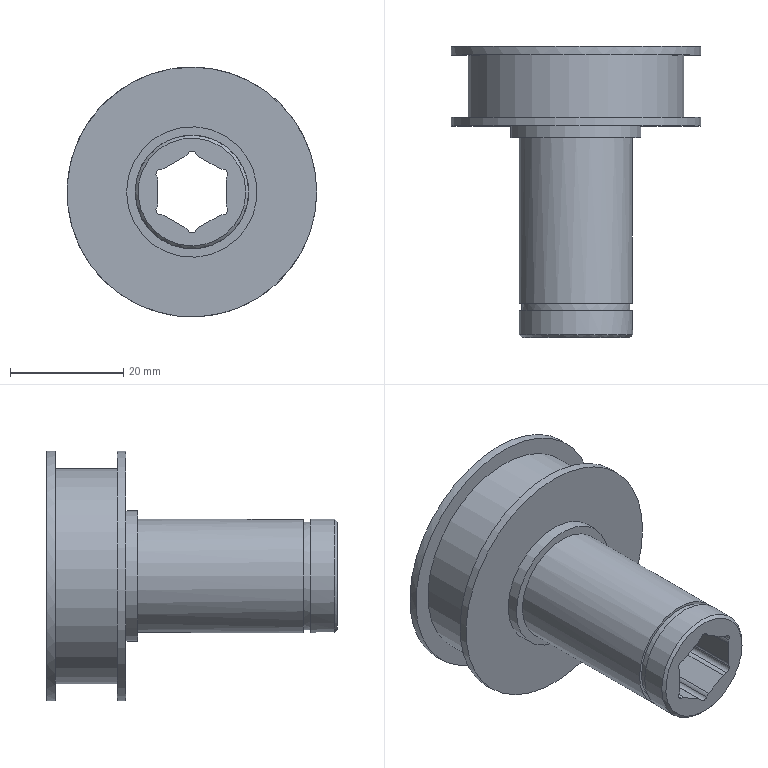Part | STEP file | ROTATION MC_NEW VER-0610_1017 | 1 solid | 40 faces | box 44 x 51.28 x 44 mm | volume 22323 mm3 | cylinder 25 | plane 14 | cone 1 | commonest cylinder face diameters 2.97 x12 1.53 x6 20 x2 44 x2 19 x1 23 x1
STEP:
#1=CARTESIAN_POINT('',(-232.469,307.008,-64.091));
#2=VERTEX_POINT('',#1);
#3=CARTESIAN_POINT('',(-210.469,307.008,-86.091));
#4=VERTEX_POINT('',#3);
#5=CARTESIAN_POINT('',(-232.469,307.008,-86.091));
#6=DIRECTION('',(0.,1.,0.));
#7=DIRECTION('',(0.,0.,1.));
#8=AXIS2_PLACEMENT_3D('',#5,#6,#7);
#9=CIRCLE('',#8,22.);
#10=EDGE_CURVE('',#2,#4,#9,.F.);
#11=ORIENTED_EDGE('',*,*,#10,.F.);
#12=CARTESIAN_POINT('',(-232.469,307.008,-86.091));
#13=DIRECTION('',(0.,1.,0.));
#14=DIRECTION('',(0.,0.,1.));
#15=AXIS2_PLACEMENT_3D('',#12,#13,#14);
#16=CIRCLE('',#15,22.);
#17=EDGE_CURVE('',#4,#2,#16,.F.);
#18=ORIENTED_EDGE('',*,*,#17,.F.);
#19=EDGE_LOOP('',(#11,#18));
#20=FACE_OUTER_BOUND('',#19,.T.);
#21=CARTESIAN_POINT('',(-226.245,307.008,-83.269));
#22=VERTEX_POINT('',#21);
#23=CARTESIAN_POINT('',(-226.454,307.008,-84.029));
#24=VERTEX_POINT('',#23);
#25=CARTESIAN_POINT('',(-224.969,307.008,-84.029));
#26=DIRECTION('',(0.,1.,0.));
#27=DIRECTION('',(-0.9641,0.,0.2654));
#28=AXIS2_PLACEMENT_3D('',#25,#26,#27);
#29=CIRCLE('',#28,1.485);
#30=EDGE_CURVE('',#22,#24,#29,.F.);
#31=ORIENTED_EDGE('',*,*,#30,.F.);
#32=CARTESIAN_POINT('',(-226.913,307.008,-82.112));
#33=VERTEX_POINT('',#32);
#34=CARTESIAN_POINT('',(-226.902,307.008,-82.877));
#35=DIRECTION('',(0.,-1.,0.));
#36=DIRECTION('',(1.,0.,0.));
#37=AXIS2_PLACEMENT_3D('',#34,#35,#36);
#38=CIRCLE('',#37,0.765);
#39=EDGE_CURVE('',#33,#22,#38,.F.);
#40=ORIENTED_EDGE('',*,*,#39,.F.);
#41=CARTESIAN_POINT('',(-227.676,307.008,-81.913));
#42=VERTEX_POINT('',#41);
#43=CARTESIAN_POINT('',(-226.933,307.008,-80.627));
#44=DIRECTION('',(0.,1.,0.));
#45=DIRECTION('',(-0.2522,0.,-0.9677));
#46=AXIS2_PLACEMENT_3D('',#43,#44,#45);
#47=CIRCLE('',#46,1.485);
#48=EDGE_CURVE('',#42,#33,#47,.F.);
#49=ORIENTED_EDGE('',*,*,#48,.F.);
#50=CARTESIAN_POINT('',(-231.248,307.008,-79.851));
#51=VERTEX_POINT('',#50);
#52=CARTESIAN_POINT('',(-227.676,307.008,-81.913));
#53=DIRECTION('',(-0.866,0.,0.5));
#54=VECTOR('',#53,4.125);
#55=LINE('',#52,#54);
#56=EDGE_CURVE('',#51,#42,#55,.F.);
#57=ORIENTED_EDGE('',*,*,#56,.F.);
#58=CARTESIAN_POINT('',(-231.802,307.008,-79.29));
#59=VERTEX_POINT('',#58);
#60=CARTESIAN_POINT('',(-230.506,307.008,-78.565));
#61=DIRECTION('',(0.,1.,0.));
#62=DIRECTION('',(-0.7119,0.,-0.7023));
#63=AXIS2_PLACEMENT_3D('',#60,#61,#62);
#64=CIRCLE('',#63,1.485);
#65=EDGE_CURVE('',#59,#51,#64,.F.);
#66=ORIENTED_EDGE('',*,*,#65,.F.);
#67=CARTESIAN_POINT('',(-233.137,307.008,-79.29));
#68=VERTEX_POINT('',#67);
#69=CARTESIAN_POINT('',(-232.469,307.008,-79.663));
#70=DIRECTION('',(0.,-1.,0.));
#71=DIRECTION('',(1.,0.,0.));
#72=AXIS2_PLACEMENT_3D('',#69,#70,#71);
#73=CIRCLE('',#72,0.765);
#74=EDGE_CURVE('',#68,#59,#73,.F.);
#75=ORIENTED_EDGE('',*,*,#74,.F.);
#76=CARTESIAN_POINT('',(-233.691,307.008,-79.851));
#77=VERTEX_POINT('',#76);
#78=CARTESIAN_POINT('',(-234.433,307.008,-78.565));
#79=DIRECTION('',(0.,1.,0.));
#80=DIRECTION('',(0.7119,0.,-0.7023));
#81=AXIS2_PLACEMENT_3D('',#78,#79,#80);
#82=CIRCLE('',#81,1.485);
#83=EDGE_CURVE('',#77,#68,#82,.F.);
#84=ORIENTED_EDGE('',*,*,#83,.F.);
#85=CARTESIAN_POINT('',(-237.263,307.008,-81.913));
#86=VERTEX_POINT('',#85);
#87=CARTESIAN_POINT('',(-233.691,307.008,-79.851));
#88=DIRECTION('',(-0.866,0.,-0.5));
#89=VECTOR('',#88,4.125);
#90=LINE('',#87,#89);
#91=EDGE_CURVE('',#86,#77,#90,.F.);
#92=ORIENTED_EDGE('',*,*,#91,.F.);
#93=CARTESIAN_POINT('',(-238.026,307.008,-82.112));
#94=VERTEX_POINT('',#93);
#95=CARTESIAN_POINT('',(-238.006,307.008,-80.627));
#96=DIRECTION('',(0.,1.,0.));
#97=DIRECTION('',(0.2522,0.,-0.9677));
#98=AXIS2_PLACEMENT_3D('',#95,#96,#97);
#99=CIRCLE('',#98,1.485);
#100=EDGE_CURVE('',#94,#86,#99,.F.);
#101=ORIENTED_EDGE('',*,*,#100,.F.);
#102=CARTESIAN_POINT('',(-238.694,307.008,-83.269));
#103=VERTEX_POINT('',#102);
#104=CARTESIAN_POINT('',(-238.036,307.008,-82.877));
#105=DIRECTION('',(0.,-1.,0.));
#106=DIRECTION('',(1.,0.,0.));
#107=AXIS2_PLACEMENT_3D('',#104,#105,#106);
#108=CIRCLE('',#107,0.765);
#109=EDGE_CURVE('',#103,#94,#108,.F.);
#110=ORIENTED_EDGE('',*,*,#109,.F.);
#111=CARTESIAN_POINT('',(-238.484,307.008,-84.029));
#112=VERTEX_POINT('',#111);
#113=CARTESIAN_POINT('',(-239.969,307.008,-84.029));
#114=DIRECTION('',(0.,1.,0.));
#115=DIRECTION('',(0.9641,0.,0.2654));
#116=AXIS2_PLACEMENT_3D('',#113,#114,#115);
#117=CIRCLE('',#116,1.485);
#118=EDGE_CURVE('',#112,#103,#117,.F.);
#119=ORIENTED_EDGE('',*,*,#118,.F.);
#120=CARTESIAN_POINT('',(-238.484,307.008,-88.154));
#121=VERTEX_POINT('',#120);
#122=CARTESIAN_POINT('',(-238.484,307.008,-84.029));
#123=DIRECTION('',(0.,0.,-1.));
#124=VECTOR('',#123,4.125);
#125=LINE('',#122,#124);
#126=EDGE_CURVE('',#121,#112,#125,.F.);
#127=ORIENTED_EDGE('',*,*,#126,.F.);
#128=CARTESIAN_POINT('',(-238.694,307.008,-88.914));
#129=VERTEX_POINT('',#128);
#130=CARTESIAN_POINT('',(-239.969,307.008,-88.154));
#131=DIRECTION('',(0.,1.,0.));
#132=DIRECTION('',(0.9641,0.,-0.2654));
#133=AXIS2_PLACEMENT_3D('',#130,#131,#132);
#134=CIRCLE('',#133,1.485);
#135=EDGE_CURVE('',#129,#121,#134,.F.);
#136=ORIENTED_EDGE('',*,*,#135,.F.);
#137=CARTESIAN_POINT('',(-238.026,307.008,-90.07));
#138=VERTEX_POINT('',#137);
#139=CARTESIAN_POINT('',(-238.036,307.008,-89.305));
#140=DIRECTION('',(0.,-1.,0.));
#141=DIRECTION('',(1.,0.,0.));
#142=AXIS2_PLACEMENT_3D('',#139,#140,#141);
#143=CIRCLE('',#142,0.765);
#144=EDGE_CURVE('',#138,#129,#143,.F.);
#145=ORIENTED_EDGE('',*,*,#144,.F.);
#146=CARTESIAN_POINT('',(-237.263,307.008,-90.269));
#147=VERTEX_POINT('',#146);
#148=CARTESIAN_POINT('',(-238.006,307.008,-91.555));
#149=DIRECTION('',(0.,1.,0.));
#150=DIRECTION('',(0.2522,0.,0.9677));
#151=AXIS2_PLACEMENT_3D('',#148,#149,#150);
#152=CIRCLE('',#151,1.485);
#153=EDGE_CURVE('',#147,#138,#152,.F.);
#154=ORIENTED_EDGE('',*,*,#153,.F.);
#155=CARTESIAN_POINT('',(-233.691,307.008,-92.332));
#156=VERTEX_POINT('',#155);
#157=CARTESIAN_POINT('',(-237.263,307.008,-90.269));
#158=DIRECTION('',(0.866,0.,-0.5));
#159=VECTOR('',#158,4.125);
#160=LINE('',#157,#159);
#161=EDGE_CURVE('',#156,#147,#160,.F.);
#162=ORIENTED_EDGE('',*,*,#161,.F.);
#163=CARTESIAN_POINT('',(-233.137,307.008,-92.893));
#164=VERTEX_POINT('',#163);
#165=CARTESIAN_POINT('',(-234.433,307.008,-93.618));
#166=DIRECTION('',(0.,1.,0.));
#167=DIRECTION('',(0.7119,0.,0.7023));
#168=AXIS2_PLACEMENT_3D('',#165,#166,#167);
#169=CIRCLE('',#168,1.485);
#170=EDGE_CURVE('',#164,#156,#169,.F.);
#171=ORIENTED_EDGE('',*,*,#170,.F.);
#172=CARTESIAN_POINT('',(-231.802,307.008,-92.893));
#173=VERTEX_POINT('',#172);
#174=CARTESIAN_POINT('',(-232.469,307.008,-92.519));
#175=DIRECTION('',(0.,-1.,0.));
#176=DIRECTION('',(1.,0.,0.));
#177=AXIS2_PLACEMENT_3D('',#174,#175,#176);
#178=CIRCLE('',#177,0.765);
#179=EDGE_CURVE('',#173,#164,#178,.F.);
#180=ORIENTED_EDGE('',*,*,#179,.F.);
#181=CARTESIAN_POINT('',(-231.248,307.008,-92.332));
#182=VERTEX_POINT('',#181);
#183=CARTESIAN_POINT('',(-230.506,307.008,-93.618));
#184=DIRECTION('',(0.,1.,0.));
#185=DIRECTION('',(-0.7119,0.,0.7023));
#186=AXIS2_PLACEMENT_3D('',#183,#184,#185);
#187=CIRCLE('',#186,1.485);
#188=EDGE_CURVE('',#182,#173,#187,.F.);
#189=ORIENTED_EDGE('',*,*,#188,.F.);
#190=CARTESIAN_POINT('',(-227.676,307.008,-90.269));
#191=VERTEX_POINT('',#190);
#192=CARTESIAN_POINT('',(-231.248,307.008,-92.332));
#193=DIRECTION('',(0.866,0.,0.5));
#194=VECTOR('',#193,4.125);
#195=LINE('',#192,#194);
#196=EDGE_CURVE('',#191,#182,#195,.F.);
#197=ORIENTED_EDGE('',*,*,#196,.F.);
#198=CARTESIAN_POINT('',(-226.913,307.008,-90.07));
#199=VERTEX_POINT('',#198);
#200=CARTESIAN_POINT('',(-226.933,307.008,-91.555));
#201=DIRECTION('',(0.,1.,0.));
#202=DIRECTION('',(-0.2522,0.,0.9677));
#203=AXIS2_PLACEMENT_3D('',#200,#201,#202);
#204=CIRCLE('',#203,1.485);
#205=EDGE_CURVE('',#199,#191,#204,.F.);
#206=ORIENTED_EDGE('',*,*,#205,.F.);
#207=CARTESIAN_POINT('',(-226.245,307.008,-88.914));
#208=VERTEX_POINT('',#207);
#209=CARTESIAN_POINT('',(-226.902,307.008,-89.305));
#210=DIRECTION('',(0.,-1.,0.));
#211=DIRECTION('',(1.,0.,0.));
#212=AXIS2_PLACEMENT_3D('',#209,#210,#211);
#213=CIRCLE('',#212,0.765);
#214=EDGE_CURVE('',#208,#199,#213,.F.);
#215=ORIENTED_EDGE('',*,*,#214,.F.);
#216=CARTESIAN_POINT('',(-226.454,307.008,-88.154));
#217=VERTEX_POINT('',#216);
#218=CARTESIAN_POINT('',(-224.969,307.008,-88.154));
#219=DIRECTION('',(0.,1.,0.));
#220=DIRECTION('',(-0.9641,0.,-0.2654));
#221=AXIS2_PLACEMENT_3D('',#218,#219,#220);
#222=CIRCLE('',#221,1.485);
#223=EDGE_CURVE('',#217,#208,#222,.F.);
#224=ORIENTED_EDGE('',*,*,#223,.F.);
#225=CARTESIAN_POINT('',(-226.454,307.008,-88.154));
#226=DIRECTION('',(0.,0.,1.));
#227=VECTOR('',#226,4.125);
#228=LINE('',#225,#227);
#229=EDGE_CURVE('',#24,#217,#228,.F.);
#230=ORIENTED_EDGE('',*,*,#229,.F.);
#231=EDGE_LOOP('',(#31,#40,#49,#57,#66,#75,#84,#92,#101,#110,#119,#127,#136,#145,#154,#162,#171,#180,#189,#197,#206,#215,#224,#230));
#232=FACE_BOUND('',#231,.T.);
#233=CARTESIAN_POINT('',(-233.469,307.008,-56.281));
#234=DIRECTION('',(0.,1.,0.));
#235=DIRECTION('',(0.,0.,1.));
#236=AXIS2_PLACEMENT_3D('',#233,#234,#235);
#237=PLANE('',#236);
#238=ADVANCED_FACE('',(#20,#232),#237,.T.);
#239=CARTESIAN_POINT('',(-237.263,255.728,-81.913));
#240=VERTEX_POINT('',#239);
#241=CARTESIAN_POINT('',(-237.263,255.728,-81.913));
#242=DIRECTION('',(0.,1.,0.));
#243=VECTOR('',#242,51.28);
#244=LINE('',#241,#243);
#245=EDGE_CURVE('',#86,#240,#244,.F.);
#246=ORIENTED_EDGE('',*,*,#245,.F.);
#247=ORIENTED_EDGE('',*,*,#91,.T.);
#248=CARTESIAN_POINT('',(-233.691,255.728,-79.851));
#249=VERTEX_POINT('',#248);
#250=CARTESIAN_POINT('',(-233.691,307.008,-79.851));
#251=DIRECTION('',(0.,-1.,0.));
#252=VECTOR('',#251,51.28);
#253=LINE('',#250,#252);
#254=EDGE_CURVE('',#249,#77,#253,.F.);
#255=ORIENTED_EDGE('',*,*,#254,.F.);
#256=CARTESIAN_POINT('',(-237.263,255.728,-81.913));
#257=DIRECTION('',(0.866,0.,0.5));
#258=VECTOR('',#257,4.125);
#259=LINE('',#256,#258);
#260=EDGE_CURVE('',#249,#240,#259,.F.);
#261=ORIENTED_EDGE('',*,*,#260,.T.);
#262=EDGE_LOOP('',(#246,#247,#255,#261));
#263=FACE_OUTER_BOUND('',#262,.T.);
#264=CARTESIAN_POINT('',(-235.477,306.008,-80.882));
#265=DIRECTION('',(0.5,0.,-0.866));
#266=DIRECTION('',(-0.866,0.,-0.5));
#267=AXIS2_PLACEMENT_3D('',#264,#265,#266);
#268=PLANE('',#267);
#269=ADVANCED_FACE('',(#263),#268,.T.);
#270=CARTESIAN_POINT('',(-233.137,255.728,-79.29));
#271=VERTEX_POINT('',#270);
#272=CARTESIAN_POINT('',(-233.137,255.728,-79.29));
#273=DIRECTION('',(0.,1.,0.));
#274=VECTOR('',#273,51.28);
#275=LINE('',#272,#274);
#276=EDGE_CURVE('',#68,#271,#275,.F.);
#277=ORIENTED_EDGE('',*,*,#276,.F.);
#278=ORIENTED_EDGE('',*,*,#74,.T.);
#279=CARTESIAN_POINT('',(-231.802,255.728,-79.29));
#280=VERTEX_POINT('',#279);
#281=CARTESIAN_POINT('',(-231.802,307.008,-79.29));
#282=DIRECTION('',(0.,-1.,0.));
#283=VECTOR('',#282,51.28);
#284=LINE('',#281,#283);
#285=EDGE_CURVE('',#280,#59,#284,.F.);
#286=ORIENTED_EDGE('',*,*,#285,.F.);
#287=CARTESIAN_POINT('',(-232.469,255.728,-79.663));
#288=DIRECTION('',(0.,1.,0.));
#289=DIRECTION('',(1.,0.,0.));
#290=AXIS2_PLACEMENT_3D('',#287,#288,#289);
#291=CIRCLE('',#290,0.765);
#292=EDGE_CURVE('',#280,#271,#291,.F.);
#293=ORIENTED_EDGE('',*,*,#292,.T.);
#294=EDGE_LOOP('',(#277,#278,#286,#293));
#295=FACE_OUTER_BOUND('',#294,.T.);
#296=CARTESIAN_POINT('',(-232.469,306.008,-79.663));
#297=DIRECTION('',(0.,1.,0.));
#298=DIRECTION('',(-1.,0.,0.));
#299=AXIS2_PLACEMENT_3D('',#296,#297,#298);
#300=CYLINDRICAL_SURFACE('',#299,0.765);
#301=ADVANCED_FACE('',(#295),#300,.F.);
#302=CARTESIAN_POINT('',(-238.484,255.728,-88.154));
#303=VERTEX_POINT('',#302);
#304=CARTESIAN_POINT('',(-238.484,255.728,-88.154));
#305=DIRECTION('',(0.,1.,0.));
#306=VECTOR('',#305,51.28);
#307=LINE('',#304,#306);
#308=EDGE_CURVE('',#121,#303,#307,.F.);
#309=ORIENTED_EDGE('',*,*,#308,.F.);
#310=ORIENTED_EDGE('',*,*,#126,.T.);
#311=CARTESIAN_POINT('',(-238.484,255.728,-84.029));
#312=VERTEX_POINT('',#311);
#313=CARTESIAN_POINT('',(-238.484,307.008,-84.029));
#314=DIRECTION('',(0.,-1.,0.));
#315=VECTOR('',#314,51.28);
#316=LINE('',#313,#315);
#317=EDGE_CURVE('',#312,#112,#316,.F.);
#318=ORIENTED_EDGE('',*,*,#317,.F.);
#319=CARTESIAN_POINT('',(-238.484,255.728,-88.154));
#320=DIRECTION('',(0.,0.,1.));
#321=VECTOR('',#320,4.125);
#322=LINE('',#319,#321);
#323=EDGE_CURVE('',#312,#303,#322,.F.);
#324=ORIENTED_EDGE('',*,*,#323,.T.);
#325=EDGE_LOOP('',(#309,#310,#318,#324));
#326=FACE_OUTER_BOUND('',#325,.T.);
#327=CARTESIAN_POINT('',(-238.484,306.008,-86.091));
#328=DIRECTION('',(1.,0.,0.));
#329=DIRECTION('',(0.,0.,-1.));
#330=AXIS2_PLACEMENT_3D('',#327,#328,#329);
#331=PLANE('',#330);
#332=ADVANCED_FACE('',(#326),#331,.T.);
#333=CARTESIAN_POINT('',(-231.248,255.728,-79.851));
#334=VERTEX_POINT('',#333);
#335=CARTESIAN_POINT('',(-231.248,255.728,-79.851));
#336=DIRECTION('',(0.,1.,0.));
#337=VECTOR('',#336,51.28);
#338=LINE('',#335,#337);
#339=EDGE_CURVE('',#51,#334,#338,.F.);
#340=ORIENTED_EDGE('',*,*,#339,.F.);
#341=ORIENTED_EDGE('',*,*,#56,.T.);
#342=CARTESIAN_POINT('',(-227.676,255.728,-81.913));
#343=VERTEX_POINT('',#342);
#344=CARTESIAN_POINT('',(-227.676,307.008,-81.913));
#345=DIRECTION('',(0.,-1.,0.));
#346=VECTOR('',#345,51.28);
#347=LINE('',#344,#346);
#348=EDGE_CURVE('',#343,#42,#347,.F.);
#349=ORIENTED_EDGE('',*,*,#348,.F.);
#350=CARTESIAN_POINT('',(-231.248,255.728,-79.851));
#351=DIRECTION('',(0.866,0.,-0.5));
#352=VECTOR('',#351,4.125);
#353=LINE('',#350,#352);
#354=EDGE_CURVE('',#343,#334,#353,.F.);
#355=ORIENTED_EDGE('',*,*,#354,.T.);
#356=EDGE_LOOP('',(#340,#341,#349,#355));
#357=FACE_OUTER_BOUND('',#356,.T.);
#358=CARTESIAN_POINT('',(-229.462,306.008,-80.882));
#359=DIRECTION('',(-0.5,0.,-0.866));
#360=DIRECTION('',(-0.866,0.,0.5));
#361=AXIS2_PLACEMENT_3D('',#358,#359,#360);
#362=PLANE('',#361);
#363=ADVANCED_FACE('',(#357),#362,.T.);
#364=CARTESIAN_POINT('',(-233.691,255.728,-92.332));
#365=VERTEX_POINT('',#364);
#366=CARTESIAN_POINT('',(-233.691,255.728,-92.332));
#367=DIRECTION('',(0.,1.,0.));
#368=VECTOR('',#367,51.28);
#369=LINE('',#366,#368);
#370=EDGE_CURVE('',#156,#365,#369,.F.);
#371=ORIENTED_EDGE('',*,*,#370,.F.);
#372=ORIENTED_EDGE('',*,*,#161,.T.);
#373=CARTESIAN_POINT('',(-237.263,255.728,-90.269));
#374=VERTEX_POINT('',#373);
#375=CARTESIAN_POINT('',(-237.263,307.008,-90.269));
#376=DIRECTION('',(0.,-1.,0.));
#377=VECTOR('',#376,51.28);
#378=LINE('',#375,#377);
#379=EDGE_CURVE('',#374,#147,#378,.F.);
#380=ORIENTED_EDGE('',*,*,#379,.F.);
#381=CARTESIAN_POINT('',(-233.691,255.728,-92.332));
#382=DIRECTION('',(-0.866,0.,0.5));
#383=VECTOR('',#382,4.125);
#384=LINE('',#381,#383);
#385=EDGE_CURVE('',#374,#365,#384,.F.);
#386=ORIENTED_EDGE('',*,*,#385,.T.);
#387=EDGE_LOOP('',(#371,#372,#380,#386));
#388=FACE_OUTER_BOUND('',#387,.T.);
#389=CARTESIAN_POINT('',(-235.477,306.008,-91.3));
#390=DIRECTION('',(0.5,0.,0.866));
#391=DIRECTION('',(0.866,0.,-0.5));
#392=AXIS2_PLACEMENT_3D('',#389,#390,#391);
#393=PLANE('',#392);
#394=ADVANCED_FACE('',(#388),#393,.T.);
#395=CARTESIAN_POINT('',(-226.454,255.728,-84.029));
#396=VERTEX_POINT('',#395);
#397=CARTESIAN_POINT('',(-226.454,255.728,-84.029));
#398=DIRECTION('',(0.,1.,0.));
#399=VECTOR('',#398,51.28);
#400=LINE('',#397,#399);
#401=EDGE_CURVE('',#24,#396,#400,.F.);
#402=ORIENTED_EDGE('',*,*,#401,.F.);
#403=ORIENTED_EDGE('',*,*,#229,.T.);
#404=CARTESIAN_POINT('',(-226.454,255.728,-88.154));
#405=VERTEX_POINT('',#404);
#406=CARTESIAN_POINT('',(-226.454,307.008,-88.154));
#407=DIRECTION('',(0.,-1.,0.));
#408=VECTOR('',#407,51.28);
#409=LINE('',#406,#408);
#410=EDGE_CURVE('',#405,#217,#409,.F.);
#411=ORIENTED_EDGE('',*,*,#410,.F.);
#412=CARTESIAN_POINT('',(-226.454,255.728,-84.029));
#413=DIRECTION('',(0.,0.,-1.));
#414=VECTOR('',#413,4.125);
#415=LINE('',#412,#414);
#416=EDGE_CURVE('',#405,#396,#415,.F.);
#417=ORIENTED_EDGE('',*,*,#416,.T.);
#418=EDGE_LOOP('',(#402,#403,#411,#417));
#419=FACE_OUTER_BOUND('',#418,.T.);
#420=CARTESIAN_POINT('',(-226.454,306.008,-86.091));
#421=DIRECTION('',(-1.,0.,0.));
#422=DIRECTION('',(0.,0.,1.));
#423=AXIS2_PLACEMENT_3D('',#420,#421,#422);
#424=PLANE('',#423);
#425=ADVANCED_FACE('',(#419),#424,.T.);
#426=CARTESIAN_POINT('',(-231.802,255.728,-92.893));
#427=VERTEX_POINT('',#426);
#428=CARTESIAN_POINT('',(-231.802,255.728,-92.893));
#429=DIRECTION('',(0.,1.,0.));
#430=VECTOR('',#429,51.28);
#431=LINE('',#428,#430);
#432=EDGE_CURVE('',#173,#427,#431,.F.);
#433=ORIENTED_EDGE('',*,*,#432,.F.);
#434=ORIENTED_EDGE('',*,*,#179,.T.);
#435=CARTESIAN_POINT('',(-233.137,255.728,-92.893));
#436=VERTEX_POINT('',#435);
#437=CARTESIAN_POINT('',(-233.137,307.008,-92.893));
#438=DIRECTION('',(0.,-1.,0.));
#439=VECTOR('',#438,51.28);
#440=LINE('',#437,#439);
#441=EDGE_CURVE('',#436,#164,#440,.F.);
#442=ORIENTED_EDGE('',*,*,#441,.F.);
#443=CARTESIAN_POINT('',(-232.469,255.728,-92.519));
#444=DIRECTION('',(0.,1.,0.));
#445=DIRECTION('',(1.,0.,0.));
#446=AXIS2_PLACEMENT_3D('',#443,#444,#445);
#447=CIRCLE('',#446,0.765);
#448=EDGE_CURVE('',#436,#427,#447,.F.);
#449=ORIENTED_EDGE('',*,*,#448,.T.);
#450=EDGE_LOOP('',(#433,#434,#442,#449));
#451=FACE_OUTER_BOUND('',#450,.T.);
#452=CARTESIAN_POINT('',(-232.469,306.008,-92.519));
#453=DIRECTION('',(0.,1.,0.));
#454=DIRECTION('',(-1.,0.,0.));
#455=AXIS2_PLACEMENT_3D('',#452,#453,#454);
#456=CYLINDRICAL_SURFACE('',#455,0.765);
#457=ADVANCED_FACE('',(#451),#456,.F.);
#458=CARTESIAN_POINT('',(-227.676,255.728,-90.269));
#459=VERTEX_POINT('',#458);
#460=CARTESIAN_POINT('',(-227.676,255.728,-90.269));
#461=DIRECTION('',(0.,1.,0.));
#462=VECTOR('',#461,51.28);
#463=LINE('',#460,#462);
#464=EDGE_CURVE('',#191,#459,#463,.F.);
#465=ORIENTED_EDGE('',*,*,#464,.F.);
#466=ORIENTED_EDGE('',*,*,#196,.T.);
#467=CARTESIAN_POINT('',(-231.248,255.728,-92.332));
#468=VERTEX_POINT('',#467);
#469=CARTESIAN_POINT('',(-231.248,307.008,-92.332));
#470=DIRECTION('',(0.,-1.,0.));
#471=VECTOR('',#470,51.28);
#472=LINE('',#469,#471);
#473=EDGE_CURVE('',#468,#182,#472,.F.);
#474=ORIENTED_EDGE('',*,*,#473,.F.);
#475=CARTESIAN_POINT('',(-227.676,255.728,-90.269));
#476=DIRECTION('',(-0.866,0.,-0.5));
#477=VECTOR('',#476,4.125);
#478=LINE('',#475,#477);
#479=EDGE_CURVE('',#468,#459,#478,.F.);
#480=ORIENTED_EDGE('',*,*,#479,.T.);
#481=EDGE_LOOP('',(#465,#466,#474,#480));
#482=FACE_OUTER_BOUND('',#481,.T.);
#483=CARTESIAN_POINT('',(-229.462,306.008,-91.3));
#484=DIRECTION('',(-0.5,0.,0.866));
#485=DIRECTION('',(0.866,0.,0.5));
#486=AXIS2_PLACEMENT_3D('',#483,#484,#485);
#487=PLANE('',#486);
#488=ADVANCED_FACE('',(#482),#487,.T.);
#489=CARTESIAN_POINT('',(-243.969,290.968,-86.091));
#490=VERTEX_POINT('',#489);
#491=CARTESIAN_POINT('',(-232.469,290.968,-86.091));
#492=DIRECTION('',(0.,-1.,0.));
#493=DIRECTION('',(-1.,0.,0.));
#494=AXIS2_PLACEMENT_3D('',#491,#492,#493);
#495=CIRCLE('',#494,11.5);
#496=EDGE_CURVE('',#490,#490,#495,.F.);
#497=ORIENTED_EDGE('',*,*,#496,.F.);
#498=EDGE_LOOP('',(#497));
#499=FACE_OUTER_BOUND('',#498,.T.);
#500=CARTESIAN_POINT('',(-232.469,290.968,-76.091));
#501=VERTEX_POINT('',#500);
#502=CARTESIAN_POINT('',(-242.469,290.968,-86.091));
#503=VERTEX_POINT('',#502);
#504=CARTESIAN_POINT('',(-232.469,290.968,-86.091));
#505=DIRECTION('',(0.,-1.,0.));
#506=DIRECTION('',(0.,0.,1.));
#507=AXIS2_PLACEMENT_3D('',#504,#505,#506);
#508=CIRCLE('',#507,10.);
#509=EDGE_CURVE('',#501,#503,#508,.F.);
#510=ORIENTED_EDGE('',*,*,#509,.T.);
#511=CARTESIAN_POINT('',(-232.469,290.968,-86.091));
#512=DIRECTION('',(0.,-1.,0.));
#513=DIRECTION('',(0.,0.,1.));
#514=AXIS2_PLACEMENT_3D('',#511,#512,#513);
#515=CIRCLE('',#514,10.);
#516=EDGE_CURVE('',#503,#501,#515,.F.);
#517=ORIENTED_EDGE('',*,*,#516,.T.);
#518=EDGE_LOOP('',(#510,#517));
#519=FACE_BOUND('',#518,.T.);
#520=CARTESIAN_POINT('',(-233.469,290.968,-56.281));
#521=DIRECTION('',(0.,1.,0.));
#522=DIRECTION('',(0.,0.,1.));
#523=AXIS2_PLACEMENT_3D('',#520,#521,#522);
#524=PLANE('',#523);
#525=ADVANCED_FACE('',(#499,#519),#524,.F.);
#526=CARTESIAN_POINT('',(-232.469,293.008,-64.091));
#527=VERTEX_POINT('',#526);
#528=CARTESIAN_POINT('',(-210.469,293.008,-86.091));
#529=VERTEX_POINT('',#528);
#530=CARTESIAN_POINT('',(-232.469,293.008,-86.091));
#531=DIRECTION('',(0.,-1.,0.));
#532=DIRECTION('',(0.,0.,1.));
#533=AXIS2_PLACEMENT_3D('',#530,#531,#532);
#534=CIRCLE('',#533,22.);
#535=EDGE_CURVE('',#527,#529,#534,.F.);
#536=ORIENTED_EDGE('',*,*,#535,.F.);
#537=CARTESIAN_POINT('',(-232.469,293.008,-86.091));
#538=DIRECTION('',(0.,-1.,0.));
#539=DIRECTION('',(0.,0.,1.));
#540=AXIS2_PLACEMENT_3D('',#537,#538,#539);
#541=CIRCLE('',#540,22.);
#542=EDGE_CURVE('',#529,#527,#541,.F.);
#543=ORIENTED_EDGE('',*,*,#542,.F.);
#544=EDGE_LOOP('',(#536,#543));
#545=FACE_OUTER_BOUND('',#544,.T.);
#546=CARTESIAN_POINT('',(-243.969,293.008,-86.091));
#547=VERTEX_POINT('',#546);
#548=CARTESIAN_POINT('',(-232.469,293.008,-86.091));
#549=DIRECTION('',(0.,-1.,0.));
#550=DIRECTION('',(-1.,0.,0.));
#551=AXIS2_PLACEMENT_3D('',#548,#549,#550);
#552=CIRCLE('',#551,11.5);
#553=EDGE_CURVE('',#547,#547,#552,.F.);
#554=ORIENTED_EDGE('',*,*,#553,.T.);
#555=EDGE_LOOP('',(#554));
#556=FACE_BOUND('',#555,.T.);
#557=CARTESIAN_POINT('',(-233.469,293.008,-56.281));
#558=DIRECTION('',(0.,1.,0.));
#559=DIRECTION('',(0.,0.,1.));
#560=AXIS2_PLACEMENT_3D('',#557,#558,#559);
#561=PLANE('',#560);
#562=ADVANCED_FACE('',(#545,#556),#561,.F.);
#563=CARTESIAN_POINT('',(-232.469,305.508,-108.091));
#564=VERTEX_POINT('',#563);
#565=CARTESIAN_POINT('',(-210.469,305.508,-86.091));
#566=VERTEX_POINT('',#565);
#567=CARTESIAN_POINT('',(-232.469,305.508,-86.091));
#568=DIRECTION('',(0.,-1.,0.));
#569=DIRECTION('',(0.,0.,-1.));
#570=AXIS2_PLACEMENT_3D('',#567,#568,#569);
#571=CIRCLE('',#570,22.);
#572=EDGE_CURVE('',#564,#566,#571,.F.);
#573=ORIENTED_EDGE('',*,*,#572,.F.);
#574=CARTESIAN_POINT('',(-232.469,305.508,-86.091));
#575=DIRECTION('',(0.,-1.,0.));
#576=DIRECTION('',(0.,0.,-1.));
#577=AXIS2_PLACEMENT_3D('',#574,#575,#576);
#578=CIRCLE('',#577,22.);
#579=EDGE_CURVE('',#566,#564,#578,.F.);
#580=ORIENTED_EDGE('',*,*,#579,.F.);
#581=EDGE_LOOP('',(#573,#580));
#582=FACE_OUTER_BOUND('',#581,.T.);
#583=CARTESIAN_POINT('',(-232.469,305.508,-105.091));
#584=VERTEX_POINT('',#583);
#585=CARTESIAN_POINT('',(-213.469,305.508,-86.091));
#586=VERTEX_POINT('',#585);
#587=CARTESIAN_POINT('',(-232.469,305.508,-86.091));
#588=DIRECTION('',(0.,1.,0.));
#589=DIRECTION('',(0.,0.,-1.));
#590=AXIS2_PLACEMENT_3D('',#587,#588,#589);
#591=CIRCLE('',#590,19.);
#592=EDGE_CURVE('',#584,#586,#591,.F.);
#593=ORIENTED_EDGE('',*,*,#592,.F.);
#594=CARTESIAN_POINT('',(-232.469,305.508,-86.091));
#595=DIRECTION('',(0.,1.,0.));
#596=DIRECTION('',(0.,0.,-1.));
#597=AXIS2_PLACEMENT_3D('',#594,#595,#596);
#598=CIRCLE('',#597,19.);
#599=EDGE_CURVE('',#586,#584,#598,.F.);
#600=ORIENTED_EDGE('',*,*,#599,.F.);
#601=EDGE_LOOP('',(#593,#600));
#602=FACE_BOUND('',#601,.T.);
#603=CARTESIAN_POINT('',(-212.469,305.508,-86.091));
#604=DIRECTION('',(0.,-1.,0.));
#605=DIRECTION('',(0.,0.,-1.));
#606=AXIS2_PLACEMENT_3D('',#603,#604,#605);
#607=PLANE('',#606);
#608=ADVANCED_FACE('',(#582,#602),#607,.T.);
#609=CARTESIAN_POINT('',(-232.469,294.508,-64.091));
#610=VERTEX_POINT('',#609);
#611=CARTESIAN_POINT('',(-210.469,294.508,-86.091));
#612=VERTEX_POINT('',#611);
#613=CARTESIAN_POINT('',(-232.469,294.508,-86.091));
#614=DIRECTION('',(0.,1.,0.));
#615=DIRECTION('',(0.,0.,1.));
#616=AXIS2_PLACEMENT_3D('',#613,#614,#615);
#617=CIRCLE('',#616,22.);
#618=EDGE_CURVE('',#610,#612,#617,.F.);
#619=ORIENTED_EDGE('',*,*,#618,.F.);
#620=CARTESIAN_POINT('',(-232.469,294.508,-86.091));
#621=DIRECTION('',(0.,1.,0.));
#622=DIRECTION('',(0.,0.,1.));
#623=AXIS2_PLACEMENT_3D('',#620,#621,#622);
#624=CIRCLE('',#623,22.);
#625=EDGE_CURVE('',#612,#610,#624,.F.);
#626=ORIENTED_EDGE('',*,*,#625,.F.);
#627=EDGE_LOOP('',(#619,#626));
#628=FACE_OUTER_BOUND('',#627,.T.);
#629=CARTESIAN_POINT('',(-232.469,294.508,-105.091));
#630=VERTEX_POINT('',#629);
#631=CARTESIAN_POINT('',(-213.469,294.508,-86.091));
#632=VERTEX_POINT('',#631);
#633=CARTESIAN_POINT('',(-232.469,294.508,-86.091));
#634=DIRECTION('',(0.,-1.,0.));
#635=DIRECTION('',(0.,0.,1.));
#636=AXIS2_PLACEMENT_3D('',#633,#634,#635);
#637=CIRCLE('',#636,19.);
#638=EDGE_CURVE('',#630,#632,#637,.F.);
#639=ORIENTED_EDGE('',*,*,#638,.F.);
#640=CARTESIAN_POINT('',(-232.469,294.508,-86.091));
#641=DIRECTION('',(0.,-1.,0.));
#642=DIRECTION('',(0.,0.,1.));
#643=AXIS2_PLACEMENT_3D('',#640,#641,#642);
#644=CIRCLE('',#643,19.);
#645=EDGE_CURVE('',#632,#630,#644,.F.);
#646=ORIENTED_EDGE('',*,*,#645,.F.);
#647=EDGE_LOOP('',(#639,#646));
#648=FACE_BOUND('',#647,.T.);
#649=CARTESIAN_POINT('',(-212.469,294.508,-86.091));
#650=DIRECTION('',(0.,1.,0.));
#651=DIRECTION('',(0.,0.,1.));
#652=AXIS2_PLACEMENT_3D('',#649,#650,#651);
#653=PLANE('',#652);
#654=ADVANCED_FACE('',(#628,#648),#653,.T.);
#655=CARTESIAN_POINT('',(-232.469,261.768,-96.091));
#656=VERTEX_POINT('',#655);
#657=CARTESIAN_POINT('',(-242.469,261.768,-86.091));
#658=VERTEX_POINT('',#657);
#659=CARTESIAN_POINT('',(-232.469,261.768,-86.091));
#660=DIRECTION('',(0.,1.,0.));
#661=DIRECTION('',(0.,0.,-1.));
#662=AXIS2_PLACEMENT_3D('',#659,#660,#661);
#663=CIRCLE('',#662,10.);
#664=EDGE_CURVE('',#656,#658,#663,.F.);
#665=ORIENTED_EDGE('',*,*,#664,.T.);
#666=CARTESIAN_POINT('',(-232.469,261.768,-86.091));
#667=DIRECTION('',(0.,1.,0.));
#668=DIRECTION('',(0.,0.,-1.));
#669=AXIS2_PLACEMENT_3D('',#666,#667,#668);
#670=CIRCLE('',#669,10.);
#671=EDGE_CURVE('',#658,#656,#670,.F.);
#672=ORIENTED_EDGE('',*,*,#671,.T.);
#673=EDGE_LOOP('',(#665,#672));
#674=FACE_OUTER_BOUND('',#673,.T.);
#675=CARTESIAN_POINT('',(-232.469,261.768,-95.591));
#676=VERTEX_POINT('',#675);
#677=CARTESIAN_POINT('',(-241.969,261.768,-86.091));
#678=VERTEX_POINT('',#677);
#679=CARTESIAN_POINT('',(-232.469,261.768,-86.091));
#680=DIRECTION('',(0.,1.,0.));
#681=DIRECTION('',(0.,0.,-1.));
#682=AXIS2_PLACEMENT_3D('',#679,#680,#681);
#683=CIRCLE('',#682,9.5);
#684=EDGE_CURVE('',#676,#678,#683,.F.);
#685=ORIENTED_EDGE('',*,*,#684,.F.);
#686=CARTESIAN_POINT('',(-232.469,261.768,-86.091));
#687=DIRECTION('',(0.,1.,0.));
#688=DIRECTION('',(0.,0.,-1.));
#689=AXIS2_PLACEMENT_3D('',#686,#687,#688);
#690=CIRCLE('',#689,9.5);
#691=EDGE_CURVE('',#678,#676,#690,.F.);
#692=ORIENTED_EDGE('',*,*,#691,.F.);
#693=EDGE_LOOP('',(#685,#692));
#694=FACE_BOUND('',#693,.T.);
#695=CARTESIAN_POINT('',(-242.469,261.768,-86.091));
#696=DIRECTION('',(0.,-1.,0.));
#697=DIRECTION('',(0.,0.,-1.));
#698=AXIS2_PLACEMENT_3D('',#695,#696,#697);
#699=PLANE('',#698);
#700=ADVANCED_FACE('',(#674,#694),#699,.T.);
#701=CARTESIAN_POINT('',(-232.469,260.468,-76.091));
#702=VERTEX_POINT('',#701);
#703=CARTESIAN_POINT('',(-242.469,260.468,-86.091));
#704=VERTEX_POINT('',#703);
#705=CARTESIAN_POINT('',(-232.469,260.468,-86.091));
#706=DIRECTION('',(0.,1.,0.));
#707=DIRECTION('',(0.,0.,1.));
#708=AXIS2_PLACEMENT_3D('',#705,#706,#707);
#709=CIRCLE('',#708,10.);
#710=EDGE_CURVE('',#702,#704,#709,.F.);
#711=ORIENTED_EDGE('',*,*,#710,.F.);
#712=CARTESIAN_POINT('',(-232.469,260.468,-86.091));
#713=DIRECTION('',(0.,1.,0.));
#714=DIRECTION('',(0.,0.,1.));
#715=AXIS2_PLACEMENT_3D('',#712,#713,#714);
#716=CIRCLE('',#715,10.);
#717=EDGE_CURVE('',#704,#702,#716,.F.);
#718=ORIENTED_EDGE('',*,*,#717,.F.);
#719=EDGE_LOOP('',(#711,#718));
#720=FACE_OUTER_BOUND('',#719,.T.);
#721=CARTESIAN_POINT('',(-232.469,260.468,-76.591));
#722=VERTEX_POINT('',#721);
#723=CARTESIAN_POINT('',(-241.969,260.468,-86.091));
#724=VERTEX_POINT('',#723);
#725=CARTESIAN_POINT('',(-232.469,260.468,-86.091));
#726=DIRECTION('',(0.,1.,0.));
#727=DIRECTION('',(0.,0.,1.));
#728=AXIS2_PLACEMENT_3D('',#725,#726,#727);
#729=CIRCLE('',#728,9.5);
#730=EDGE_CURVE('',#722,#724,#729,.F.);
#731=ORIENTED_EDGE('',*,*,#730,.T.);
#732=CARTESIAN_POINT('',(-232.469,260.468,-86.091));
#733=DIRECTION('',(0.,1.,0.));
#734=DIRECTION('',(0.,0.,1.));
#735=AXIS2_PLACEMENT_3D('',#732,#733,#734);
#736=CIRCLE('',#735,9.5);
#737=EDGE_CURVE('',#724,#722,#736,.F.);
#738=ORIENTED_EDGE('',*,*,#737,.T.);
#739=EDGE_LOOP('',(#731,#738));
#740=FACE_BOUND('',#739,.T.);
#741=CARTESIAN_POINT('',(-242.469,260.468,-86.091));
#742=DIRECTION('',(0.,1.,0.));
#743=DIRECTION('',(0.,0.,1.));
#744=AXIS2_PLACEMENT_3D('',#741,#742,#743);
#745=PLANE('',#744);
#746=ADVANCED_FACE('',(#720,#740),#745,.T.);
#747=CARTESIAN_POINT('',(-232.469,255.728,-95.591));
#748=VERTEX_POINT('',#747);
#749=CARTESIAN_POINT('',(-222.969,255.728,-86.091));
#750=VERTEX_POINT('',#749);
#751=CARTESIAN_POINT('',(-232.469,255.728,-86.091));
#752=DIRECTION('',(0.,-1.,0.));
#753=DIRECTION('',(0.,0.,-1.));
#754=AXIS2_PLACEMENT_3D('',#751,#752,#753);
#755=CIRCLE('',#754,9.5);
#756=EDGE_CURVE('',#748,#750,#755,.F.);
#757=ORIENTED_EDGE('',*,*,#756,.F.);
#758=CARTESIAN_POINT('',(-232.469,255.728,-86.091));
#759=DIRECTION('',(0.,-1.,0.));
#760=DIRECTION('',(0.,0.,-1.));
#761=AXIS2_PLACEMENT_3D('',#758,#759,#760);
#762=CIRCLE('',#761,9.5);
#763=EDGE_CURVE('',#750,#748,#762,.F.);
#764=ORIENTED_EDGE('',*,*,#763,.F.);
#765=EDGE_LOOP('',(#757,#764));
#766=FACE_OUTER_BOUND('',#765,.T.);
#767=CARTESIAN_POINT('',(-238.694,255.728,-88.914));
#768=VERTEX_POINT('',#767);
#769=CARTESIAN_POINT('',(-238.026,255.728,-90.07));
#770=VERTEX_POINT('',#769);
#771=CARTESIAN_POINT('',(-238.036,255.728,-89.305));
#772=DIRECTION('',(0.,1.,0.));
#773=DIRECTION('',(1.,0.,0.));
#774=AXIS2_PLACEMENT_3D('',#771,#772,#773);
#775=CIRCLE('',#774,0.765);
#776=EDGE_CURVE('',#768,#770,#775,.F.);
#777=ORIENTED_EDGE('',*,*,#776,.F.);
#778=CARTESIAN_POINT('',(-239.969,255.728,-88.154));
#779=DIRECTION('',(0.,-1.,0.));
#780=DIRECTION('',(0.9641,0.,-0.2654));
#781=AXIS2_PLACEMENT_3D('',#778,#779,#780);
#782=CIRCLE('',#781,1.485);
#783=EDGE_CURVE('',#303,#768,#782,.F.);
#784=ORIENTED_EDGE('',*,*,#783,.F.);
#785=ORIENTED_EDGE('',*,*,#323,.F.);
#786=CARTESIAN_POINT('',(-238.694,255.728,-83.269));
#787=VERTEX_POINT('',#786);
#788=CARTESIAN_POINT('',(-239.969,255.728,-84.029));
#789=DIRECTION('',(0.,-1.,0.));
#790=DIRECTION('',(0.9641,0.,0.2654));
#791=AXIS2_PLACEMENT_3D('',#788,#789,#790);
#792=CIRCLE('',#791,1.485);
#793=EDGE_CURVE('',#787,#312,#792,.F.);
#794=ORIENTED_EDGE('',*,*,#793,.F.);
#795=CARTESIAN_POINT('',(-238.026,255.728,-82.112));
#796=VERTEX_POINT('',#795);
#797=CARTESIAN_POINT('',(-238.036,255.728,-82.877));
#798=DIRECTION('',(0.,1.,0.));
#799=DIRECTION('',(1.,0.,0.));
#800=AXIS2_PLACEMENT_3D('',#797,#798,#799);
#801=CIRCLE('',#800,0.765);
#802=EDGE_CURVE('',#796,#787,#801,.F.);
#803=ORIENTED_EDGE('',*,*,#802,.F.);
#804=CARTESIAN_POINT('',(-238.006,255.728,-80.627));
#805=DIRECTION('',(0.,-1.,0.));
#806=DIRECTION('',(0.2522,0.,-0.9677));
#807=AXIS2_PLACEMENT_3D('',#804,#805,#806);
#808=CIRCLE('',#807,1.485);
#809=EDGE_CURVE('',#240,#796,#808,.F.);
#810=ORIENTED_EDGE('',*,*,#809,.F.);
#811=ORIENTED_EDGE('',*,*,#260,.F.);
#812=CARTESIAN_POINT('',(-234.433,255.728,-78.565));
#813=DIRECTION('',(0.,-1.,0.));
#814=DIRECTION('',(0.7119,0.,-0.7023));
#815=AXIS2_PLACEMENT_3D('',#812,#813,#814);
#816=CIRCLE('',#815,1.485);
#817=EDGE_CURVE('',#271,#249,#816,.F.);
#818=ORIENTED_EDGE('',*,*,#817,.F.);
#819=ORIENTED_EDGE('',*,*,#292,.F.);
#820=CARTESIAN_POINT('',(-230.506,255.728,-78.565));
#821=DIRECTION('',(0.,-1.,0.));
#822=DIRECTION('',(-0.7119,0.,-0.7023));
#823=AXIS2_PLACEMENT_3D('',#820,#821,#822);
#824=CIRCLE('',#823,1.485);
#825=EDGE_CURVE('',#334,#280,#824,.F.);
#826=ORIENTED_EDGE('',*,*,#825,.F.);
#827=ORIENTED_EDGE('',*,*,#354,.F.);
#828=CARTESIAN_POINT('',(-226.913,255.728,-82.112));
#829=VERTEX_POINT('',#828);
#830=CARTESIAN_POINT('',(-226.933,255.728,-80.627));
#831=DIRECTION('',(0.,-1.,0.));
#832=DIRECTION('',(-0.2522,0.,-0.9677));
#833=AXIS2_PLACEMENT_3D('',#830,#831,#832);
#834=CIRCLE('',#833,1.485);
#835=EDGE_CURVE('',#829,#343,#834,.F.);
#836=ORIENTED_EDGE('',*,*,#835,.F.);
#837=CARTESIAN_POINT('',(-226.245,255.728,-83.269));
#838=VERTEX_POINT('',#837);
#839=CARTESIAN_POINT('',(-226.902,255.728,-82.877));
#840=DIRECTION('',(0.,1.,0.));
#841=DIRECTION('',(1.,0.,0.));
#842=AXIS2_PLACEMENT_3D('',#839,#840,#841);
#843=CIRCLE('',#842,0.765);
#844=EDGE_CURVE('',#838,#829,#843,.F.);
#845=ORIENTED_EDGE('',*,*,#844,.F.);
#846=CARTESIAN_POINT('',(-224.969,255.728,-84.029));
#847=DIRECTION('',(0.,-1.,0.));
#848=DIRECTION('',(-0.9641,0.,0.2654));
#849=AXIS2_PLACEMENT_3D('',#846,#847,#848);
#850=CIRCLE('',#849,1.485);
#851=EDGE_CURVE('',#396,#838,#850,.F.);
#852=ORIENTED_EDGE('',*,*,#851,.F.);
#853=ORIENTED_EDGE('',*,*,#416,.F.);
#854=CARTESIAN_POINT('',(-226.245,255.728,-88.914));
#855=VERTEX_POINT('',#854);
#856=CARTESIAN_POINT('',(-224.969,255.728,-88.154));
#857=DIRECTION('',(0.,-1.,0.));
#858=DIRECTION('',(-0.9641,0.,-0.2654));
#859=AXIS2_PLACEMENT_3D('',#856,#857,#858);
#860=CIRCLE('',#859,1.485);
#861=EDGE_CURVE('',#855,#405,#860,.F.);
#862=ORIENTED_EDGE('',*,*,#861,.F.);
#863=CARTESIAN_POINT('',(-226.913,255.728,-90.07));
#864=VERTEX_POINT('',#863);
#865=CARTESIAN_POINT('',(-226.902,255.728,-89.305));
#866=DIRECTION('',(0.,1.,0.));
#867=DIRECTION('',(1.,0.,0.));
#868=AXIS2_PLACEMENT_3D('',#865,#866,#867);
#869=CIRCLE('',#868,0.765);
#870=EDGE_CURVE('',#864,#855,#869,.F.);
#871=ORIENTED_EDGE('',*,*,#870,.F.);
#872=CARTESIAN_POINT('',(-226.933,255.728,-91.555));
#873=DIRECTION('',(0.,-1.,0.));
#874=DIRECTION('',(-0.2522,0.,0.9677));
#875=AXIS2_PLACEMENT_3D('',#872,#873,#874);
#876=CIRCLE('',#875,1.485);
#877=EDGE_CURVE('',#459,#864,#876,.F.);
#878=ORIENTED_EDGE('',*,*,#877,.F.);
#879=ORIENTED_EDGE('',*,*,#479,.F.);
#880=CARTESIAN_POINT('',(-230.506,255.728,-93.618));
#881=DIRECTION('',(0.,-1.,0.));
#882=DIRECTION('',(-0.7119,0.,0.7023));
#883=AXIS2_PLACEMENT_3D('',#880,#881,#882);
#884=CIRCLE('',#883,1.485);
#885=EDGE_CURVE('',#427,#468,#884,.F.);
#886=ORIENTED_EDGE('',*,*,#885,.F.);
#887=ORIENTED_EDGE('',*,*,#448,.F.);
#888=CARTESIAN_POINT('',(-234.433,255.728,-93.618));
#889=DIRECTION('',(0.,-1.,0.));
#890=DIRECTION('',(0.7119,0.,0.7023));
#891=AXIS2_PLACEMENT_3D('',#888,#889,#890);
#892=CIRCLE('',#891,1.485);
#893=EDGE_CURVE('',#365,#436,#892,.F.);
#894=ORIENTED_EDGE('',*,*,#893,.F.);
#895=ORIENTED_EDGE('',*,*,#385,.F.);
#896=CARTESIAN_POINT('',(-238.006,255.728,-91.555));
#897=DIRECTION('',(0.,-1.,0.));
#898=DIRECTION('',(0.2522,0.,0.9677));
#899=AXIS2_PLACEMENT_3D('',#896,#897,#898);
#900=CIRCLE('',#899,1.485);
#901=EDGE_CURVE('',#770,#374,#900,.F.);
#902=ORIENTED_EDGE('',*,*,#901,.F.);
#903=EDGE_LOOP('',(#777,#784,#785,#794,#803,#810,#811,#818,#819,#826,#827,#836,#845,#852,#853,#862,#871,#878,#879,#886,#887,#894,#895,#902));
#904=FACE_BOUND('',#903,.T.);
#905=CARTESIAN_POINT('',(-232.469,255.728,-86.091));
#906=DIRECTION('',(0.,-1.,0.));
#907=DIRECTION('',(0.,0.,-1.));
#908=AXIS2_PLACEMENT_3D('',#905,#906,#907);
#909=PLANE('',#908);
#910=ADVANCED_FACE('',(#766,#904),#909,.T.);
#911=ORIENTED_EDGE('',*,*,#205,.T.);
#912=ORIENTED_EDGE('',*,*,#464,.T.);
#913=ORIENTED_EDGE('',*,*,#877,.T.);
#914=CARTESIAN_POINT('',(-226.913,307.008,-90.07));
#915=DIRECTION('',(0.,-1.,0.));
#916=VECTOR('',#915,51.28);
#917=LINE('',#914,#916);
#918=EDGE_CURVE('',#864,#199,#917,.F.);
#919=ORIENTED_EDGE('',*,*,#918,.T.);
#920=EDGE_LOOP('',(#911,#912,#913,#919));
#921=FACE_OUTER_BOUND('',#920,.T.);
#922=CARTESIAN_POINT('',(-226.933,306.008,-91.555));
#923=DIRECTION('',(0.,1.,0.));
#924=DIRECTION('',(-0.2522,0.,0.9677));
#925=AXIS2_PLACEMENT_3D('',#922,#923,#924);
#926=CYLINDRICAL_SURFACE('',#925,1.485);
#927=ADVANCED_FACE('',(#921),#926,.T.);
#928=ORIENTED_EDGE('',*,*,#885,.T.);
#929=ORIENTED_EDGE('',*,*,#473,.T.);
#930=ORIENTED_EDGE('',*,*,#188,.T.);
#931=ORIENTED_EDGE('',*,*,#432,.T.);
#932=EDGE_LOOP('',(#928,#929,#930,#931));
#933=FACE_OUTER_BOUND('',#932,.T.);
#934=CARTESIAN_POINT('',(-230.506,306.008,-93.618));
#935=DIRECTION('',(0.,-1.,0.));
#936=DIRECTION('',(-0.7119,0.,0.7023));
#937=AXIS2_PLACEMENT_3D('',#934,#935,#936);
#938=CYLINDRICAL_SURFACE('',#937,1.485);
#939=ADVANCED_FACE('',(#933),#938,.T.);
#940=ORIENTED_EDGE('',*,*,#214,.T.);
#941=ORIENTED_EDGE('',*,*,#918,.F.);
#942=ORIENTED_EDGE('',*,*,#870,.T.);
#943=CARTESIAN_POINT('',(-226.245,255.728,-88.914));
#944=DIRECTION('',(0.,1.,0.));
#945=VECTOR('',#944,51.28);
#946=LINE('',#943,#945);
#947=EDGE_CURVE('',#208,#855,#946,.F.);
#948=ORIENTED_EDGE('',*,*,#947,.F.);
#949=EDGE_LOOP('',(#940,#941,#942,#948));
#950=FACE_OUTER_BOUND('',#949,.T.);
#951=CARTESIAN_POINT('',(-226.902,306.008,-89.305));
#952=DIRECTION('',(0.,1.,0.));
#953=DIRECTION('',(0.866,0.,-0.5));
#954=AXIS2_PLACEMENT_3D('',#951,#952,#953);
#955=CYLINDRICAL_SURFACE('',#954,0.765);
#956=ADVANCED_FACE('',(#950),#955,.F.);
#957=ORIENTED_EDGE('',*,*,#861,.T.);
#958=ORIENTED_EDGE('',*,*,#410,.T.);
#959=ORIENTED_EDGE('',*,*,#223,.T.);
#960=ORIENTED_EDGE('',*,*,#947,.T.);
#961=EDGE_LOOP('',(#957,#958,#959,#960));
#962=FACE_OUTER_BOUND('',#961,.T.);
#963=CARTESIAN_POINT('',(-224.969,306.008,-88.154));
#964=DIRECTION('',(0.,-1.,0.));
#965=DIRECTION('',(-0.9641,0.,-0.2654));
#966=AXIS2_PLACEMENT_3D('',#963,#964,#965);
#967=CYLINDRICAL_SURFACE('',#966,1.485);
#968=ADVANCED_FACE('',(#962),#967,.T.);
#969=ORIENTED_EDGE('',*,*,#170,.T.);
#970=ORIENTED_EDGE('',*,*,#370,.T.);
#971=ORIENTED_EDGE('',*,*,#893,.T.);
#972=ORIENTED_EDGE('',*,*,#441,.T.);
#973=EDGE_LOOP('',(#969,#970,#971,#972));
#974=FACE_OUTER_BOUND('',#973,.T.);
#975=CARTESIAN_POINT('',(-234.433,306.008,-93.618));
#976=DIRECTION('',(0.,1.,0.));
#977=DIRECTION('',(0.7119,0.,0.7023));
#978=AXIS2_PLACEMENT_3D('',#975,#976,#977);
#979=CYLINDRICAL_SURFACE('',#978,1.485);
#980=ADVANCED_FACE('',(#974),#979,.T.);
#981=ORIENTED_EDGE('',*,*,#30,.T.);
#982=ORIENTED_EDGE('',*,*,#401,.T.);
#983=ORIENTED_EDGE('',*,*,#851,.T.);
#984=CARTESIAN_POINT('',(-226.245,307.008,-83.269));
#985=DIRECTION('',(0.,-1.,0.));
#986=VECTOR('',#985,51.28);
#987=LINE('',#984,#986);
#988=EDGE_CURVE('',#838,#22,#987,.F.);
#989=ORIENTED_EDGE('',*,*,#988,.T.);
#990=EDGE_LOOP('',(#981,#982,#983,#989));
#991=FACE_OUTER_BOUND('',#990,.T.);
#992=CARTESIAN_POINT('',(-224.969,306.008,-84.029));
#993=DIRECTION('',(0.,1.,0.));
#994=DIRECTION('',(-0.9641,0.,0.2654));
#995=AXIS2_PLACEMENT_3D('',#992,#993,#994);
#996=CYLINDRICAL_SURFACE('',#995,1.485);
#997=ADVANCED_FACE('',(#991),#996,.T.);
#998=ORIENTED_EDGE('',*,*,#901,.T.);
#999=ORIENTED_EDGE('',*,*,#379,.T.);
#1000=ORIENTED_EDGE('',*,*,#153,.T.);
#1001=CARTESIAN_POINT('',(-238.026,255.728,-90.07));
#1002=DIRECTION('',(0.,1.,0.));
#1003=VECTOR('',#1002,51.28);
#1004=LINE('',#1001,#1003);
#1005=EDGE_CURVE('',#138,#770,#1004,.F.);
#1006=ORIENTED_EDGE('',*,*,#1005,.T.);
#1007=EDGE_LOOP('',(#998,#999,#1000,#1006));
#1008=FACE_OUTER_BOUND('',#1007,.T.);
#1009=CARTESIAN_POINT('',(-238.006,306.008,-91.555));
#1010=DIRECTION('',(0.,-1.,0.));
#1011=DIRECTION('',(0.2522,0.,0.9677));
#1012=AXIS2_PLACEMENT_3D('',#1009,#1010,#1011);
#1013=CYLINDRICAL_SURFACE('',#1012,1.485);
#1014=ADVANCED_FACE('',(#1008),#1013,.T.);
#1015=ORIENTED_EDGE('',*,*,#39,.T.);
#1016=ORIENTED_EDGE('',*,*,#988,.F.);
#1017=ORIENTED_EDGE('',*,*,#844,.T.);
#1018=CARTESIAN_POINT('',(-226.913,255.728,-82.112));
#1019=DIRECTION('',(0.,1.,0.));
#1020=VECTOR('',#1019,51.28);
#1021=LINE('',#1018,#1020);
#1022=EDGE_CURVE('',#33,#829,#1021,.F.);
#1023=ORIENTED_EDGE('',*,*,#1022,.F.);
#1024=EDGE_LOOP('',(#1015,#1016,#1017,#1023));
#1025=FACE_OUTER_BOUND('',#1024,.T.);
#1026=CARTESIAN_POINT('',(-226.902,306.008,-82.877));
#1027=DIRECTION('',(0.,1.,0.));
#1028=DIRECTION('',(0.866,0.,0.5));
#1029=AXIS2_PLACEMENT_3D('',#1026,#1027,#1028);
#1030=CYLINDRICAL_SURFACE('',#1029,0.765);
#1031=ADVANCED_FACE('',(#1025),#1030,.F.);
#1032=ORIENTED_EDGE('',*,*,#776,.T.);
#1033=ORIENTED_EDGE('',*,*,#1005,.F.);
#1034=ORIENTED_EDGE('',*,*,#144,.T.);
#1035=CARTESIAN_POINT('',(-238.694,307.008,-88.914));
#1036=DIRECTION('',(0.,-1.,0.));
#1037=VECTOR('',#1036,51.28);
#1038=LINE('',#1035,#1037);
#1039=EDGE_CURVE('',#768,#129,#1038,.F.);
#1040=ORIENTED_EDGE('',*,*,#1039,.F.);
#1041=EDGE_LOOP('',(#1032,#1033,#1034,#1040));
#1042=FACE_OUTER_BOUND('',#1041,.T.);
#1043=CARTESIAN_POINT('',(-238.036,306.008,-89.305));
#1044=DIRECTION('',(0.,1.,0.));
#1045=DIRECTION('',(-1.,0.,0.));
#1046=AXIS2_PLACEMENT_3D('',#1043,#1044,#1045);
#1047=CYLINDRICAL_SURFACE('',#1046,0.765);
#1048=ADVANCED_FACE('',(#1042),#1047,.F.);
#1049=ORIENTED_EDGE('',*,*,#835,.T.);
#1050=ORIENTED_EDGE('',*,*,#348,.T.);
#1051=ORIENTED_EDGE('',*,*,#48,.T.);
#1052=ORIENTED_EDGE('',*,*,#1022,.T.);
#1053=EDGE_LOOP('',(#1049,#1050,#1051,#1052));
#1054=FACE_OUTER_BOUND('',#1053,.T.);
#1055=CARTESIAN_POINT('',(-226.933,306.008,-80.627));
#1056=DIRECTION('',(0.,-1.,0.));
#1057=DIRECTION('',(-0.2522,0.,-0.9677));
#1058=AXIS2_PLACEMENT_3D('',#1055,#1056,#1057);
#1059=CYLINDRICAL_SURFACE('',#1058,1.485);
#1060=ADVANCED_FACE('',(#1054),#1059,.T.);
#1061=ORIENTED_EDGE('',*,*,#135,.T.);
#1062=ORIENTED_EDGE('',*,*,#308,.T.);
#1063=ORIENTED_EDGE('',*,*,#783,.T.);
#1064=ORIENTED_EDGE('',*,*,#1039,.T.);
#1065=EDGE_LOOP('',(#1061,#1062,#1063,#1064));
#1066=FACE_OUTER_BOUND('',#1065,.T.);
#1067=CARTESIAN_POINT('',(-239.969,306.008,-88.154));
#1068=DIRECTION('',(0.,1.,0.));
#1069=DIRECTION('',(0.9641,0.,-0.2654));
#1070=AXIS2_PLACEMENT_3D('',#1067,#1068,#1069);
#1071=CYLINDRICAL_SURFACE('',#1070,1.485);
#1072=ADVANCED_FACE('',(#1066),#1071,.T.);
#1073=ORIENTED_EDGE('',*,*,#65,.T.);
#1074=ORIENTED_EDGE('',*,*,#339,.T.);
#1075=ORIENTED_EDGE('',*,*,#825,.T.);
#1076=ORIENTED_EDGE('',*,*,#285,.T.);
#1077=EDGE_LOOP('',(#1073,#1074,#1075,#1076));
#1078=FACE_OUTER_BOUND('',#1077,.T.);
#1079=CARTESIAN_POINT('',(-230.506,306.008,-78.565));
#1080=DIRECTION('',(0.,1.,0.));
#1081=DIRECTION('',(-0.7119,0.,-0.7023));
#1082=AXIS2_PLACEMENT_3D('',#1079,#1080,#1081);
#1083=CYLINDRICAL_SURFACE('',#1082,1.485);
#1084=ADVANCED_FACE('',(#1078),#1083,.T.);
#1085=ORIENTED_EDGE('',*,*,#793,.T.);
#1086=ORIENTED_EDGE('',*,*,#317,.T.);
#1087=ORIENTED_EDGE('',*,*,#118,.T.);
#1088=CARTESIAN_POINT('',(-238.694,255.728,-83.269));
#1089=DIRECTION('',(0.,1.,0.));
#1090=VECTOR('',#1089,51.28);
#1091=LINE('',#1088,#1090);
#1092=EDGE_CURVE('',#103,#787,#1091,.F.);
#1093=ORIENTED_EDGE('',*,*,#1092,.T.);
#1094=EDGE_LOOP('',(#1085,#1086,#1087,#1093));
#1095=FACE_OUTER_BOUND('',#1094,.T.);
#1096=CARTESIAN_POINT('',(-239.969,306.008,-84.029));
#1097=DIRECTION('',(0.,-1.,0.));
#1098=DIRECTION('',(0.9641,0.,0.2654));
#1099=AXIS2_PLACEMENT_3D('',#1096,#1097,#1098);
#1100=CYLINDRICAL_SURFACE('',#1099,1.485);
#1101=ADVANCED_FACE('',(#1095),#1100,.T.);
#1102=ORIENTED_EDGE('',*,*,#802,.T.);
#1103=ORIENTED_EDGE('',*,*,#1092,.F.);
#1104=ORIENTED_EDGE('',*,*,#109,.T.);
#1105=CARTESIAN_POINT('',(-238.026,307.008,-82.112));
#1106=DIRECTION('',(0.,-1.,0.));
#1107=VECTOR('',#1106,51.28);
#1108=LINE('',#1105,#1107);
#1109=EDGE_CURVE('',#796,#94,#1108,.F.);
#1110=ORIENTED_EDGE('',*,*,#1109,.F.);
#1111=EDGE_LOOP('',(#1102,#1103,#1104,#1110));
#1112=FACE_OUTER_BOUND('',#1111,.T.);
#1113=CARTESIAN_POINT('',(-238.036,306.008,-82.877));
#1114=DIRECTION('',(0.,1.,0.));
#1115=DIRECTION('',(-1.,0.,0.));
#1116=AXIS2_PLACEMENT_3D('',#1113,#1114,#1115);
#1117=CYLINDRICAL_SURFACE('',#1116,0.765);
#1118=ADVANCED_FACE('',(#1112),#1117,.F.);
#1119=ORIENTED_EDGE('',*,*,#817,.T.);
#1120=ORIENTED_EDGE('',*,*,#254,.T.);
#1121=ORIENTED_EDGE('',*,*,#83,.T.);
#1122=ORIENTED_EDGE('',*,*,#276,.T.);
#1123=EDGE_LOOP('',(#1119,#1120,#1121,#1122));
#1124=FACE_OUTER_BOUND('',#1123,.T.);
#1125=CARTESIAN_POINT('',(-234.433,306.008,-78.565));
#1126=DIRECTION('',(0.,-1.,0.));
#1127=DIRECTION('',(0.7119,0.,-0.7023));
#1128=AXIS2_PLACEMENT_3D('',#1125,#1126,#1127);
#1129=CYLINDRICAL_SURFACE('',#1128,1.485);
#1130=ADVANCED_FACE('',(#1124),#1129,.T.);
#1131=ORIENTED_EDGE('',*,*,#100,.T.);
#1132=ORIENTED_EDGE('',*,*,#245,.T.);
#1133=ORIENTED_EDGE('',*,*,#809,.T.);
#1134=ORIENTED_EDGE('',*,*,#1109,.T.);
#1135=EDGE_LOOP('',(#1131,#1132,#1133,#1134));
#1136=FACE_OUTER_BOUND('',#1135,.T.);
#1137=CARTESIAN_POINT('',(-238.006,306.008,-80.627));
#1138=DIRECTION('',(0.,1.,0.));
#1139=DIRECTION('',(0.2522,0.,-0.9677));
#1140=AXIS2_PLACEMENT_3D('',#1137,#1138,#1139);
#1141=CYLINDRICAL_SURFACE('',#1140,1.485);
#1142=ADVANCED_FACE('',(#1136),#1141,.T.);
#1143=ORIENTED_EDGE('',*,*,#592,.T.);
#1144=CARTESIAN_POINT('',(-213.469,293.508,-86.091));
#1145=DIRECTION('',(0.,-1.,0.));
#1146=VECTOR('',#1145,19.);
#1147=LINE('',#1144,#1146);
#1148=EDGE_CURVE('',#586,#632,#1147,.T.);
#1149=ORIENTED_EDGE('',*,*,#1148,.T.);
#1150=ORIENTED_EDGE('',*,*,#645,.T.);
#1151=ORIENTED_EDGE('',*,*,#638,.T.);
#1152=ORIENTED_EDGE('',*,*,#1148,.F.);
#1153=ORIENTED_EDGE('',*,*,#599,.T.);
#1154=EDGE_LOOP('',(#1143,#1149,#1150,#1151,#1152,#1153));
#1155=FACE_OUTER_BOUND('',#1154,.T.);
#1156=CARTESIAN_POINT('',(-232.469,293.508,-86.091));
#1157=DIRECTION('',(0.,1.,0.));
#1158=DIRECTION('',(-1.,0.,0.));
#1159=AXIS2_PLACEMENT_3D('',#1156,#1157,#1158);
#1160=CYLINDRICAL_SURFACE('',#1159,19.);
#1161=ADVANCED_FACE('',(#1155),#1160,.T.);
#1162=ORIENTED_EDGE('',*,*,#10,.T.);
#1163=CARTESIAN_POINT('',(-210.469,293.008,-86.091));
#1164=DIRECTION('',(0.,-1.,0.));
#1165=VECTOR('',#1164,22.);
#1166=LINE('',#1163,#1165);
#1167=EDGE_CURVE('',#4,#566,#1166,.T.);
#1168=ORIENTED_EDGE('',*,*,#1167,.T.);
#1169=ORIENTED_EDGE('',*,*,#579,.T.);
#1170=ORIENTED_EDGE('',*,*,#572,.T.);
#1171=ORIENTED_EDGE('',*,*,#1167,.F.);
#1172=ORIENTED_EDGE('',*,*,#17,.T.);
#1173=EDGE_LOOP('',(#1162,#1168,#1169,#1170,#1171,#1172));
#1174=FACE_OUTER_BOUND('',#1173,.T.);
#1175=CARTESIAN_POINT('',(-232.469,293.008,-86.091));
#1176=DIRECTION('',(0.,1.,0.));
#1177=DIRECTION('',(-1.,0.,0.));
#1178=AXIS2_PLACEMENT_3D('',#1175,#1176,#1177);
#1179=CYLINDRICAL_SURFACE('',#1178,22.);
#1180=ADVANCED_FACE('',(#1174),#1179,.T.);
#1181=ORIENTED_EDGE('',*,*,#553,.F.);
#1182=CARTESIAN_POINT('',(-243.969,293.008,-86.091));
#1183=DIRECTION('',(0.,-1.,0.));
#1184=VECTOR('',#1183,11.5);
#1185=LINE('',#1182,#1184);
#1186=EDGE_CURVE('',#547,#490,#1185,.T.);
#1187=ORIENTED_EDGE('',*,*,#1186,.T.);
#1188=ORIENTED_EDGE('',*,*,#496,.T.);
#1189=ORIENTED_EDGE('',*,*,#1186,.F.);
#1190=EDGE_LOOP('',(#1181,#1187,#1188,#1189));
#1191=FACE_OUTER_BOUND('',#1190,.T.);
#1192=CARTESIAN_POINT('',(-232.469,293.008,-86.091));
#1193=DIRECTION('',(0.,1.,0.));
#1194=DIRECTION('',(1.,0.,0.));
#1195=AXIS2_PLACEMENT_3D('',#1192,#1193,#1194);
#1196=CYLINDRICAL_SURFACE('',#1195,11.5);
#1197=ADVANCED_FACE('',(#1191),#1196,.T.);
#1198=ORIENTED_EDGE('',*,*,#618,.T.);
#1199=CARTESIAN_POINT('',(-210.469,293.008,-86.091));
#1200=DIRECTION('',(0.,-1.,0.));
#1201=VECTOR('',#1200,22.);
#1202=LINE('',#1199,#1201);
#1203=EDGE_CURVE('',#612,#529,#1202,.T.);
#1204=ORIENTED_EDGE('',*,*,#1203,.T.);
#1205=ORIENTED_EDGE('',*,*,#542,.T.);
#1206=ORIENTED_EDGE('',*,*,#535,.T.);
#1207=ORIENTED_EDGE('',*,*,#1203,.F.);
#1208=ORIENTED_EDGE('',*,*,#625,.T.);
#1209=EDGE_LOOP('',(#1198,#1204,#1205,#1206,#1207,#1208));
#1210=FACE_OUTER_BOUND('',#1209,.T.);
#1211=CARTESIAN_POINT('',(-232.469,293.008,-86.091));
#1212=DIRECTION('',(0.,1.,0.));
#1213=DIRECTION('',(-1.,0.,0.));
#1214=AXIS2_PLACEMENT_3D('',#1211,#1212,#1213);
#1215=CYLINDRICAL_SURFACE('',#1214,22.);
#1216=ADVANCED_FACE('',(#1210),#1215,.T.);
#1217=ORIENTED_EDGE('',*,*,#730,.F.);
#1218=ORIENTED_EDGE('',*,*,#737,.F.);
#1219=CARTESIAN_POINT('',(-241.969,303.808,-86.091));
#1220=DIRECTION('',(0.,1.,0.));
#1221=VECTOR('',#1220,9.5);
#1222=LINE('',#1219,#1221);
#1223=EDGE_CURVE('',#724,#678,#1222,.T.);
#1224=ORIENTED_EDGE('',*,*,#1223,.T.);
#1225=ORIENTED_EDGE('',*,*,#691,.T.);
#1226=ORIENTED_EDGE('',*,*,#684,.T.);
#1227=ORIENTED_EDGE('',*,*,#1223,.F.);
#1228=EDGE_LOOP('',(#1217,#1218,#1224,#1225,#1226,#1227));
#1229=FACE_OUTER_BOUND('',#1228,.T.);
#1230=CARTESIAN_POINT('',(-232.469,303.808,-86.091));
#1231=DIRECTION('',(0.,-1.,0.));
#1232=DIRECTION('',(1.,0.,0.));
#1233=AXIS2_PLACEMENT_3D('',#1230,#1231,#1232);
#1234=CYLINDRICAL_SURFACE('',#1233,9.5);
#1235=ADVANCED_FACE('',(#1229),#1234,.T.);
#1236=ORIENTED_EDGE('',*,*,#664,.F.);
#1237=ORIENTED_EDGE('',*,*,#671,.F.);
#1238=CARTESIAN_POINT('',(-242.469,293.008,-86.091));
#1239=DIRECTION('',(0.,1.,0.));
#1240=VECTOR('',#1239,10.);
#1241=LINE('',#1238,#1240);
#1242=EDGE_CURVE('',#658,#503,#1241,.T.);
#1243=ORIENTED_EDGE('',*,*,#1242,.T.);
#1244=ORIENTED_EDGE('',*,*,#509,.F.);
#1245=ORIENTED_EDGE('',*,*,#516,.F.);
#1246=ORIENTED_EDGE('',*,*,#1242,.F.);
#1247=EDGE_LOOP('',(#1236,#1237,#1243,#1244,#1245,#1246));
#1248=FACE_OUTER_BOUND('',#1247,.T.);
#1249=CARTESIAN_POINT('',(-232.469,293.008,-86.091));
#1250=DIRECTION('',(0.,-1.,0.));
#1251=DIRECTION('',(1.,0.,0.));
#1252=AXIS2_PLACEMENT_3D('',#1249,#1250,#1251);
#1253=CYLINDRICAL_SURFACE('',#1252,10.);
#1254=ADVANCED_FACE('',(#1248),#1253,.T.);
#1255=CARTESIAN_POINT('',(-232.469,256.228,-76.091));
#1256=VERTEX_POINT('',#1255);
#1257=CARTESIAN_POINT('',(-242.469,256.228,-86.091));
#1258=VERTEX_POINT('',#1257);
#1259=CARTESIAN_POINT('',(-232.469,256.228,-86.091));
#1260=DIRECTION('',(0.,1.,0.));
#1261=DIRECTION('',(0.,0.,1.));
#1262=AXIS2_PLACEMENT_3D('',#1259,#1260,#1261);
#1263=CIRCLE('',#1262,10.);
#1264=EDGE_CURVE('',#1256,#1258,#1263,.F.);
#1265=ORIENTED_EDGE('',*,*,#1264,.F.);
#1266=CARTESIAN_POINT('',(-222.469,256.228,-86.091));
#1267=VERTEX_POINT('',#1266);
#1268=CARTESIAN_POINT('',(-232.469,256.228,-86.091));
#1269=DIRECTION('',(0.,1.,0.));
#1270=DIRECTION('',(0.,0.,1.));
#1271=AXIS2_PLACEMENT_3D('',#1268,#1269,#1270);
#1272=CIRCLE('',#1271,10.);
#1273=EDGE_CURVE('',#1267,#1256,#1272,.F.);
#1274=ORIENTED_EDGE('',*,*,#1273,.F.);
#1275=CARTESIAN_POINT('',(-232.469,256.228,-86.091));
#1276=DIRECTION('',(0.,1.,0.));
#1277=DIRECTION('',(0.,0.,1.));
#1278=AXIS2_PLACEMENT_3D('',#1275,#1276,#1277);
#1279=CIRCLE('',#1278,10.);
#1280=EDGE_CURVE('',#1258,#1267,#1279,.F.);
#1281=ORIENTED_EDGE('',*,*,#1280,.F.);
#1282=CARTESIAN_POINT('',(-242.469,301.008,-86.091));
#1283=DIRECTION('',(0.,1.,0.));
#1284=VECTOR('',#1283,10.);
#1285=LINE('',#1282,#1284);
#1286=EDGE_CURVE('',#1258,#704,#1285,.T.);
#1287=ORIENTED_EDGE('',*,*,#1286,.T.);
#1288=ORIENTED_EDGE('',*,*,#717,.T.);
#1289=ORIENTED_EDGE('',*,*,#710,.T.);
#1290=ORIENTED_EDGE('',*,*,#1286,.F.);
#1291=EDGE_LOOP('',(#1265,#1274,#1281,#1287,#1288,#1289,#1290));
#1292=FACE_OUTER_BOUND('',#1291,.T.);
#1293=CARTESIAN_POINT('',(-232.469,301.008,-86.091));
#1294=DIRECTION('',(0.,-1.,0.));
#1295=DIRECTION('',(1.,0.,0.));
#1296=AXIS2_PLACEMENT_3D('',#1293,#1294,#1295);
#1297=CYLINDRICAL_SURFACE('',#1296,10.);
#1298=ADVANCED_FACE('',(#1292),#1297,.T.);
#1299=ORIENTED_EDGE('',*,*,#1264,.T.);
#1300=ORIENTED_EDGE('',*,*,#1280,.T.);
#1301=CARTESIAN_POINT('',(-222.969,255.728,-86.091));
#1302=DIRECTION('',(-0.7071,-0.7071,0.));
#1303=VECTOR('',#1302,9.5);
#1304=LINE('',#1301,#1303);
#1305=EDGE_CURVE('',#1267,#750,#1304,.T.);
#1306=ORIENTED_EDGE('',*,*,#1305,.T.);
#1307=ORIENTED_EDGE('',*,*,#763,.T.);
#1308=ORIENTED_EDGE('',*,*,#756,.T.);
#1309=ORIENTED_EDGE('',*,*,#1305,.F.);
#1310=ORIENTED_EDGE('',*,*,#1273,.T.);
#1311=EDGE_LOOP('',(#1299,#1300,#1306,#1307,#1308,#1309,#1310));
#1312=FACE_OUTER_BOUND('',#1311,.T.);
#1313=CARTESIAN_POINT('',(-232.469,255.728,-86.091));
#1314=DIRECTION('',(0.,1.,0.));
#1315=DIRECTION('',(-1.,0.,0.));
#1316=AXIS2_PLACEMENT_3D('',#1313,#1314,#1315);
#1317=CONICAL_SURFACE('',#1316,9.5,0.7854);
#1318=ADVANCED_FACE('',(#1312),#1317,.T.);
#1319=CLOSED_SHELL('',(#238,#269,#301,#332,#363,#394,#425,#457,#488,#525,#562,#608,#654,#700,#746,#910,#927,#939,#956,#968,#980,#997,#1014,#1031,#1048,#1060,#1072,#1084,#1101,#1118,#1130,#1142,#1161,#1180,#1197,#1216,#1235,#1254,#1298,#1318));
#1320=MANIFOLD_SOLID_BREP('',#1319);
#1321=(LENGTH_UNIT()NAMED_UNIT(*)SI_UNIT(.MILLI.,.METRE.));
#1322=UNCERTAINTY_MEASURE_WITH_UNIT(LENGTH_MEASURE(0.01),#1321,'','');
#1323=(NAMED_UNIT(*)PLANE_ANGLE_UNIT()SI_UNIT($,.RADIAN.));
#1324=(NAMED_UNIT(*)SI_UNIT($,.STERADIAN.)SOLID_ANGLE_UNIT());
#1325=(GEOMETRIC_REPRESENTATION_CONTEXT(3)GLOBAL_UNCERTAINTY_ASSIGNED_CONTEXT((#1322))GLOBAL_UNIT_ASSIGNED_CONTEXT((#1321,#1323,#1324))REPRESENTATION_CONTEXT('',''));
#1326=ADVANCED_BREP_SHAPE_REPRESENTATION('',(#1320),#1325);